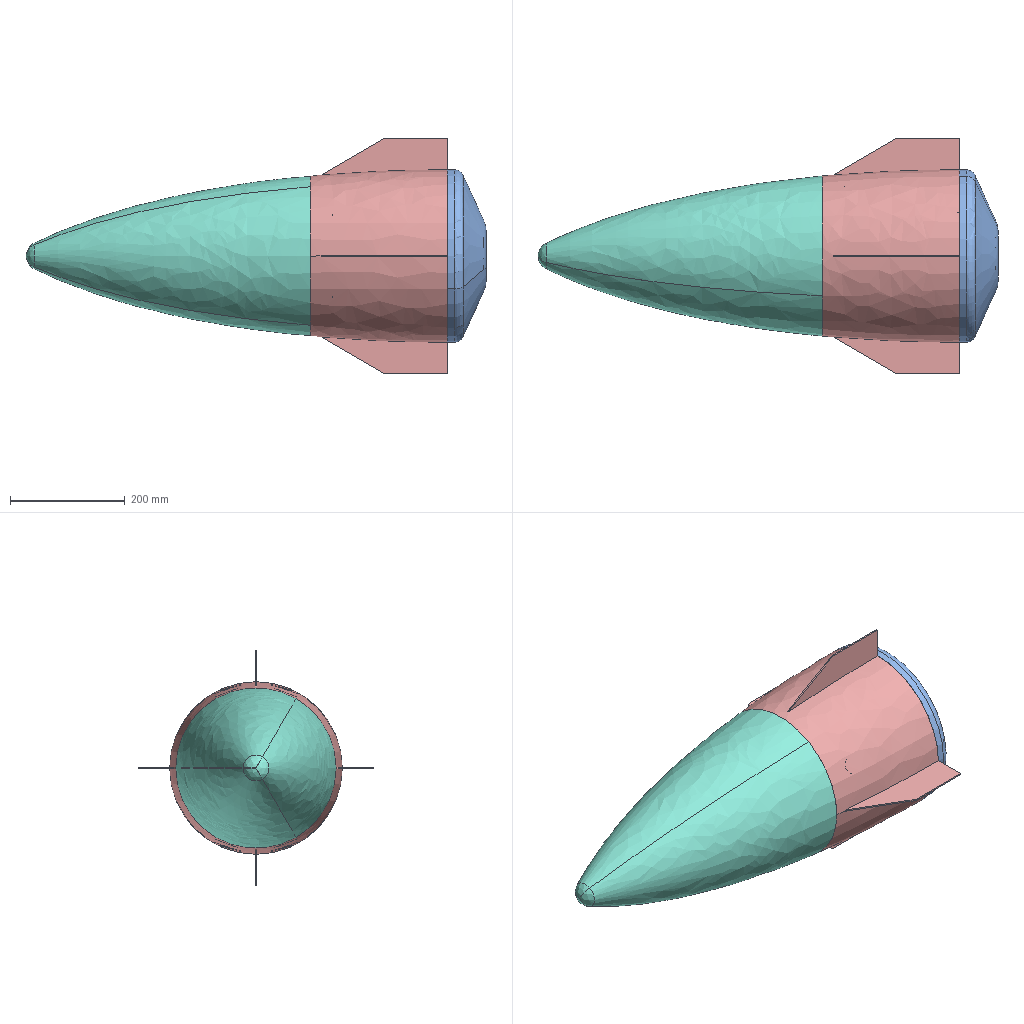Assembly | SolidWorks | 31 different items | 41 placed | box 800 x 410 x 410 mm
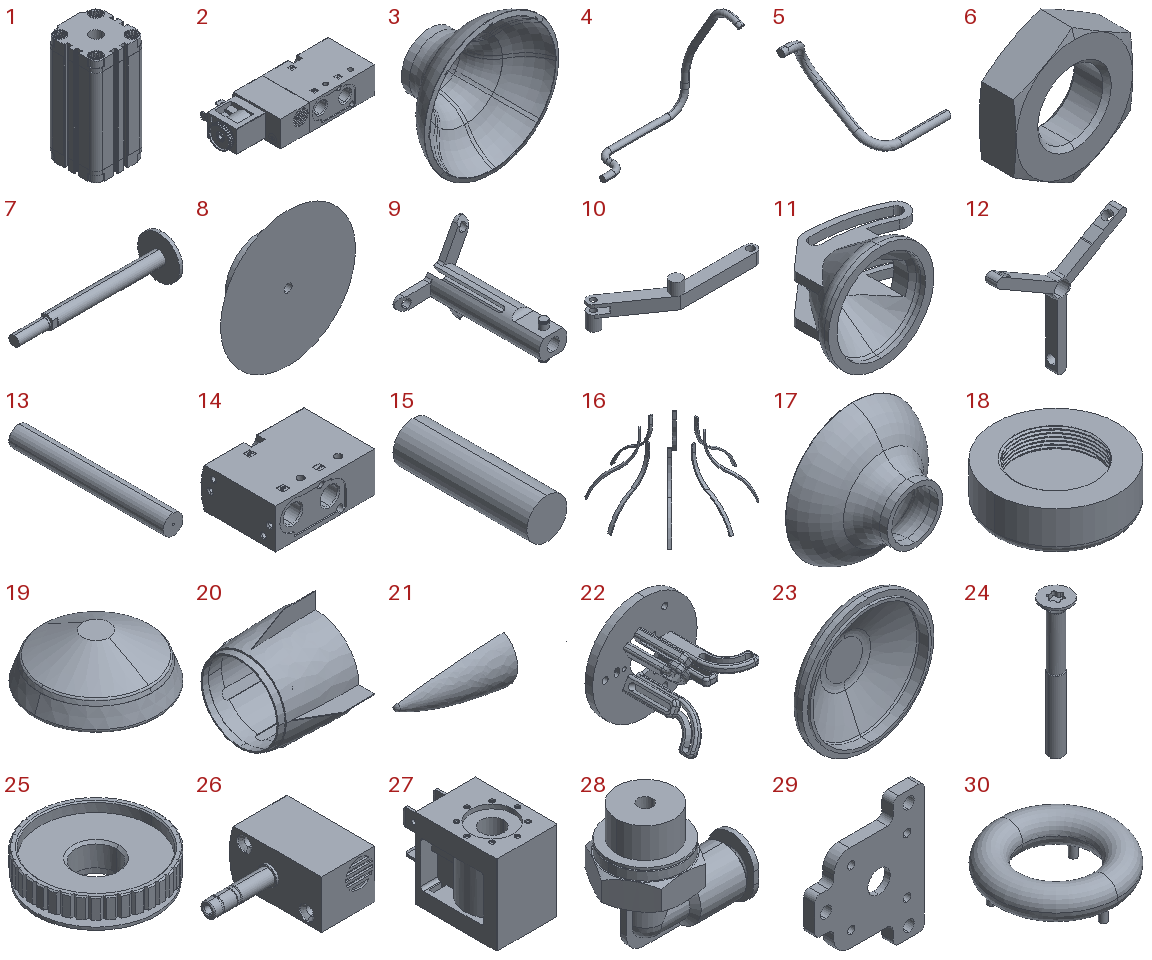Parts list (item | name | quantity | parent item | size | volume | features):
1 | (subassembly) | x1 | - | 68 x 71 x 145.5 mm | 391762 mm3 | -
2 | (subassembly) | x1 | - | 129.15 x 57.2 x 26.5 mm | 130620 mm3 | -
3 | (subassembly) | x1 | - | 209.773 x 99.35 x 209.773 mm | 365370 mm3 | -
4 | - | x1 | - | 74.439 x 42.263 x 75.178 mm | 2118 mm3 | features 3DProfileFeature 2, Sweep 1
5 | - | x1 | - | 58.57 x 42.483 x 46.069 mm | 1368 mm3 | features 3DProfileFeature 2, Sweep 1
6 | - | x1 | - | 19 x 6 x 21.939 mm | 1319 mm3 | features BaseBody 1
7 | - | x1 | - | 176 x 50 x 50 mm | 38817 mm3 | features BaseBody 1, ICE 1
8 | - | x1 | - | 30 x 6 x 30 mm | 2026 mm3 | features HoleWzd 1, Revolution 1
9 | - | x1 | - | 94.58 x 150 x 115.79 mm | 107737 mm3 | features ICE 5, Fillet 2, SweepThread 2, Chamfer 1, Cut 1, Revolution 1
10 | - | x3 | - | 181.532 x 61.886 x 48 mm | 50544 mm3 | features ICE 5, Extrusion 1
11 | - | x1 | - | 107.891 x 64.658 x 86.78 mm | 76040 mm3 | features ICE 5, MirrorPattern 1, Revolution 1
12 | - | x1 | - | 113.655 x 10 x 99.5 mm | 13029 mm3 | features CirPattern 2, Fillet 2, ICE 2, Cut 1, Extrusion 1
13 | - | x1 | - | 16 x 125 x 16 mm | 25103 mm3 | features HoleWzd 1, RevCut 1, Revolution 1
14 | - | x1 | in 2 | 66 x 50.5 x 26.5 mm | 77595 mm3 | features BaseBody 1
15 | - | x1 | - | 6 x 20 x 6 mm | 565.487 mm3 | features Extrusion 1
16 | - | x1 | in 3 | 199.946 x 199.946 x 99.301 mm | 9875 mm3 | features CirPattern 1, ICE 1
17 | - | x1 | in 3 | 209.773 x 99.35 x 209.773 mm | 355495 mm3 | features Revolution 1
18 | - | x2 | - | 15 x 15 x 5 mm | 677.673 mm3 | features ICE 2, Extrusion 1, Fillet 1, SweepThread 1
19 | - | x1 | - | 216.513 x 216.513 x 137.693 mm | 2586859 mm3 | features BaseBody 1, Revolution 1
20 | - | x1 | - | 260.298 x 410 x 410 mm | 1987551 mm3 | features ICE 3, CirPattern 2, Revolution 2, RefAxis 1
21 | - | x3 | - | 733.25 x 150.001 x 241.12 mm | 643249 mm3 | features ICE 5, Fillet 3, Revolution 3, CombineBodies 1, RefAxis 1, RevCut 1
22 | - | x1 | - | 276 x 197.346 x 276 mm | 1375608 mm3 | features ICE 11, CirPattern 4, Cut 2, Fillet 2, Extrusion 1
23 | - | x1 | - | 300 x 73 x 300 mm | 1152181 mm3 | features Fillet 4, Revolution 1
24 | - | x2 | in 2 | 7.9 x 7.9 x 37.5 mm | 495.827 mm3 | features BaseBody 1
25 | - | x1 | in 2 | 21.485 x 21.485 x 6.9 mm | 915.19 mm3 | features BaseBody 1
26 | - | x1 | in 2 | 62.1 x 49.6 x 25.9 mm | 36554 mm3 | features BaseBody 1
27 | - | x1 | in 2 | 22 x 41.7 x 29 mm | 14563 mm3 | features BaseBody 1
28 | - | x5 | - | 23.206 x 13 x 21.4 mm | 1816 mm3 | features ICE 10, Fillet 2, BaseBody 1, Chamfer 1, HoleWzd 1, RevCut 1
29 | - | x1 | - | 98 x 10 x 115 mm | 49580 mm3 | features ICE 5, Fillet 4, Cut 1, Extrusion 1
30 | - | x1 | - | 273 x 273 x 90.3 mm | 274529 mm3 | features Fillet 4, BaseBody 1, ICE 1, Scale 1
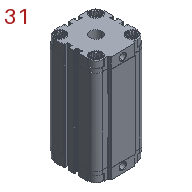31 | - | x1 | in 1 | 68 x 71 x 145.5 mm | 391762 mm3 | features BaseBody 1
Mates (type | each side: item.copy, entity, surface, feature):
In the top assembly
Coincident | 20.1 plane | 21.1 plane
Concentric | 20.1 face cylinder Revolve3 | 22.1 face cylinder Boss-Extrude1
Coincident | 20.1 plane | 22.1 plane
DistanceDim | 22.1 face plane Boss-Extrude1 | 20.1 face plane Revolve3
Coincident | 22.1 face plane Boss-Extrude2 | 10.1 face plane Boss-Extrude1
Slot | 10.1 face cylinder Boss-Extrude2 | 22.1 face cylinder Cut-Extrude5
Concentric | 21.1 face cylinder Cut-Extrude4 | 10.1 face cylinder Cut-Extrude1
Lock | 21.1 select_type:0 | 10.1 select_type:0
Concentric | 22.1 face cylinder CirPattern8 | 30.1 face cylinder Imported3 | 2 times
Coincident | 22.1 face plane Boss-Extrude1 | 30.1 face plane Imported3
Concentric | 22.1 face cylinder Cut-Extrude12 | 9.1 face cylinder Revolution1
Parallel | 22.1 face plane Boss-Extrude2 | 12.1 face plane Boss-Extrude1
Concentric | 22.1 face cylinder Cut-Extrude12 | 12.1 face cylinder Cut-Extrude4
Concentric | 10.1 face cylinder Cut-Extrude3 | 15.1 face cylinder Boss-Extrude1
Coincident | 10.1 face plane Boss-Extrude1 | 15.1 face plane Boss-Extrude1
Concentric | 15.1 face cylinder Boss-Extrude1 | 12.1 face cylinder Cut-Extrude5
Coincident | 29.1 face plane Boss-Extrude2 | 22.1 face plane Cut-Extrude14
Parallel | 29.1 face plane Boss-Extrude3 | 22.1 face plane Cut-Extrude12
Parallel | 22.1 face plane Cut-Extrude12 | 31.1 face plane Imported1
Concentric | 31.1 face cylinder Imported1 | 7.1 face cylinder Imported1
Concentric | 29.1 face cylinder Cut-Extrude1 | 7.1 face cylinder Imported1
Concentric | 22.1 face cylinder Cut-Extrude12 | 7.1 face cylinder Imported1
Coincident | 31.1 face plane Imported1 | 29.1 face plane Boss-Extrude2
Concentric | 7.1 face cylinder Imported1 | 6.1 face cylinder Imported1
Coincident | 12.1 face plane Boss-Extrude1 | 6.1 face plane Imported1
LimitDistanceDim | 7.1 face plane Imported1 | 31.1 face plane Imported1
Coincident | 14.1 face plane Imported1 | 29.1 face plane Boss-Extrude1
Coincident | 14.1 face plane Imported1 | 31.1 face plane Imported1 | 2 times
Concentric | 14.1 face cylinder Imported1 | 28.1 face cylinder Boss-Extrude5
Coincident | 14.1 face plane Imported1 | 28.1 face plane Imported3
Concentric | 14.1 face cylinder Imported1 | 28.2 face cylinder Boss-Extrude5
Coincident | 14.1 face plane Imported1 | 28.2 face plane Imported3
Concentric | 14.1 face cylinder Imported1 | 28.3 face cylinder Boss-Extrude5
Coincident | 14.1 face plane Imported1 | 28.3 face plane Imported3
Concentric | 31.1 face cylinder Imported1 | 28.4 face cylinder Boss-Extrude5
Coincident | 31.1 face plane Imported1 | 28.4 face plane Imported3
Parallel | 31.1 face plane Imported1 | 28.4 face plane Imported3
Parallel | 29.1 face plane Boss-Extrude1 | 28.1 face plane Imported3
Parallel | 29.1 face plane Boss-Extrude1 | 28.2 face plane Imported3
Parallel | 28.2 face plane Imported3 | 28.3 face plane Imported3
Concentric | 30.1 face cylinder Imported3 | 28.5 face cylinder Boss-Extrude5
Coincident | 30.1 face plane Imported3 | 28.5 face plane Imported3
Parallel | 22.1 face plane Boss-Extrude1 | 28.5 face plane Imported3
Coincident | 28.1 edge | 5.1 face cylinder Sweep1
Coincident | 28.4 edge | 5.1 face plane Sweep1
Coincident | 28.5 edge | 4.1 face cylinder Sweep1
Tangent | 28.2 face cylinder Cut-Revolve1 | 4.1 face torus Sweep1
Concentric | 20.1 face cylinder Revolve3 | 23.1 face cylinder Revolve1
Coincident | 20.1 face plane Revolve3 | 23.1 face plane Revolve1
Coincident | 17.1 face plane Revolution1 | 11.1 edge
Concentric | 17.1 face cylinder Revolution1 | 11.1 face cylinder Revolution1
Concentric | 22.1 edge | 9.1 face cylinder Revolution1
Coincident | 22.1 face plane Boss-Extrude1 | 9.1 face plane Revolution1
Coincident | 11.1 face plane Boss-Extrude1 | 9.1 face plane Cortar-Extruir2
Concentric | 9.1 face cylinder Boss-Extrude3 | 18.1 face cylinder Boss-Extrude1
Coincident | 9.1 face plane Boss-Extrude4 | 18.1 face plane Cut-Extrude1
Coincident | 9.1 face plane Boss-Extrude3 | 18.2 face plane Cut-Extrude1
Concentric | 9.1 face cylinder Boss-Extrude3 | 18.2 face cylinder Boss-Extrude1
Tangent | 11.1 face cylinder Boss-Extrude2 | 9.1 face cylinder Boss-Extrude3
Concentric | 19.1 edge | 17.1 edge
Concentric | 11.1 face cylinder Boss-Extrude2 | 9.1 face cylinder Boss-Extrude3
Concentric | 9.1 face cylinder Revolution1 | 13.1 face cylinder Revolution1
Concentric | 13.1 face cylinder Revolution1 | 8.1 face cylinder Revolution1
Coincident | 13.1 face plane Revolution1 | 8.1 face plane Revolution1
DistanceDim | 6.1 face plane Imported1 | 7.1 face plane Boss-Extrude1
Coincident | 7.1 face plane Boss-Extrude1 | 13.1 face plane Revolution1
In subassembly 3
Coincident | 16.1 face plane PatternC2 | 17.2 face plane Revolution1
Coincident | 16.1 select_type:24 | 17.2 select_type:24